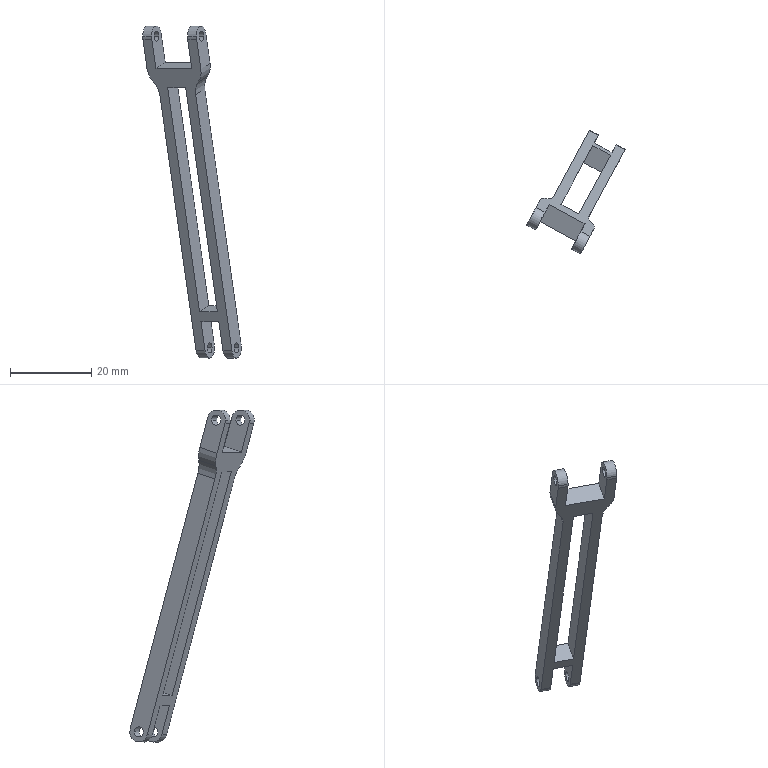Part | SolidWorks | features ICE 7, HoleWzd 4, Extrusion 1 | 1 solid | 34 faces | box 24.253 x 30.565 x 81.628 mm | volume 2325 mm3 | cylinder 18 | plane 16 | commonest cylinder face diameters 2.5 x8 5 x6 10 x4
STEP:
#1=CARTESIAN_POINT('',(-37.304,-81.964,-265.344));
#2=VERTEX_POINT('',#1);
#3=CARTESIAN_POINT('',(-38.488,-84.166,-265.344));
#4=VERTEX_POINT('',#3);
#5=CARTESIAN_POINT('',(-37.896,-83.065,-265.344));
#6=DIRECTION('',(-0.8809,0.4732,0.));
#7=DIRECTION('',(-0.4732,-0.8809,0.));
#8=AXIS2_PLACEMENT_3D('',#5,#6,#7);
#9=CIRCLE('',#8,1.25);
#10=EDGE_CURVE('',#2,#4,#9,.T.);
#11=ORIENTED_EDGE('',*,*,#10,.T.);
#12=CARTESIAN_POINT('',(-36.285,-85.349,-265.344));
#13=VERTEX_POINT('',#12);
#14=CARTESIAN_POINT('',(-36.285,-85.349,-265.344));
#15=DIRECTION('',(0.8809,-0.4732,0.));
#16=VECTOR('',#15,1000.);
#17=LINE('',#14,#16);
#18=EDGE_CURVE('',#4,#13,#17,.T.);
#19=ORIENTED_EDGE('',*,*,#18,.T.);
#20=CARTESIAN_POINT('',(-35.102,-83.147,-265.344));
#21=VERTEX_POINT('',#20);
#22=CARTESIAN_POINT('',(-35.694,-84.248,-265.344));
#23=DIRECTION('',(-0.8809,0.4732,0.));
#24=DIRECTION('',(-0.4732,-0.8809,0.));
#25=AXIS2_PLACEMENT_3D('',#22,#23,#24);
#26=CIRCLE('',#25,1.25);
#27=EDGE_CURVE('',#21,#13,#26,.T.);
#28=ORIENTED_EDGE('',*,*,#27,.F.);
#29=CARTESIAN_POINT('',(-35.102,-83.147,-265.344));
#30=DIRECTION('',(0.8809,-0.4732,0.));
#31=VECTOR('',#30,1000.);
#32=LINE('',#29,#31);
#33=EDGE_CURVE('',#2,#21,#32,.T.);
#34=ORIENTED_EDGE('',*,*,#33,.F.);
#35=EDGE_LOOP('',(#11,#19,#28,#34));
#36=FACE_OUTER_BOUND('',#35,.T.);
#37=CARTESIAN_POINT('',(-35.694,-84.248,-265.344));
#38=DIRECTION('',(0.8809,-0.4732,0.));
#39=DIRECTION('',(0.4732,0.8809,0.));
#40=AXIS2_PLACEMENT_3D('',#37,#38,#39);
#41=CYLINDRICAL_SURFACE('',#40,1.25);
#42=ADVANCED_FACE('',(#36),#41,.F.);
#43=CARTESIAN_POINT('',(-27.476,-90.082,-265.344));
#44=VERTEX_POINT('',#43);
#45=CARTESIAN_POINT('',(-26.293,-87.879,-265.344));
#46=VERTEX_POINT('',#45);
#47=CARTESIAN_POINT('',(-26.884,-88.981,-265.344));
#48=DIRECTION('',(0.8809,-0.4732,0.));
#49=DIRECTION('',(0.4732,0.8809,0.));
#50=AXIS2_PLACEMENT_3D('',#47,#48,#49);
#51=CIRCLE('',#50,1.25);
#52=EDGE_CURVE('',#44,#46,#51,.T.);
#53=ORIENTED_EDGE('',*,*,#52,.F.);
#54=CARTESIAN_POINT('',(-25.274,-91.265,-265.344));
#55=VERTEX_POINT('',#54);
#56=CARTESIAN_POINT('',(-25.274,-91.265,-265.344));
#57=DIRECTION('',(0.8809,-0.4732,0.));
#58=VECTOR('',#57,1000.);
#59=LINE('',#56,#58);
#60=EDGE_CURVE('',#44,#55,#59,.T.);
#61=ORIENTED_EDGE('',*,*,#60,.T.);
#62=CARTESIAN_POINT('',(-24.09,-89.063,-265.344));
#63=VERTEX_POINT('',#62);
#64=CARTESIAN_POINT('',(-24.682,-90.164,-265.344));
#65=DIRECTION('',(0.8809,-0.4732,0.));
#66=DIRECTION('',(0.4732,0.8809,0.));
#67=AXIS2_PLACEMENT_3D('',#64,#65,#66);
#68=CIRCLE('',#67,1.25);
#69=EDGE_CURVE('',#55,#63,#68,.T.);
#70=ORIENTED_EDGE('',*,*,#69,.T.);
#71=CARTESIAN_POINT('',(-24.09,-89.063,-265.344));
#72=DIRECTION('',(0.8809,-0.4732,0.));
#73=VECTOR('',#72,1000.);
#74=LINE('',#71,#73);
#75=EDGE_CURVE('',#46,#63,#74,.T.);
#76=ORIENTED_EDGE('',*,*,#75,.F.);
#77=EDGE_LOOP('',(#53,#61,#70,#76));
#78=FACE_OUTER_BOUND('',#77,.T.);
#79=CARTESIAN_POINT('',(-24.682,-90.164,-265.344));
#80=DIRECTION('',(0.8809,-0.4732,0.));
#81=DIRECTION('',(0.4732,0.8809,0.));
#82=AXIS2_PLACEMENT_3D('',#79,#80,#81);
#83=CYLINDRICAL_SURFACE('',#82,1.25);
#84=ADVANCED_FACE('',(#78),#83,.F.);
#85=CARTESIAN_POINT('',(-25.41,-65.105,-341.972));
#86=VERTEX_POINT('',#85);
#87=CARTESIAN_POINT('',(-24.227,-62.902,-341.972));
#88=VERTEX_POINT('',#87);
#89=CARTESIAN_POINT('',(-24.818,-64.003,-341.972));
#90=DIRECTION('',(0.8809,-0.4732,0.));
#91=DIRECTION('',(0.4732,0.8809,0.));
#92=AXIS2_PLACEMENT_3D('',#89,#90,#91);
#93=CIRCLE('',#92,1.25);
#94=EDGE_CURVE('',#86,#88,#93,.T.);
#95=ORIENTED_EDGE('',*,*,#94,.F.);
#96=CARTESIAN_POINT('',(-23.207,-66.288,-341.972));
#97=VERTEX_POINT('',#96);
#98=CARTESIAN_POINT('',(-23.207,-66.288,-341.972));
#99=DIRECTION('',(0.8809,-0.4732,0.));
#100=VECTOR('',#99,1000.);
#101=LINE('',#98,#100);
#102=EDGE_CURVE('',#86,#97,#101,.T.);
#103=ORIENTED_EDGE('',*,*,#102,.T.);
#104=CARTESIAN_POINT('',(-22.024,-64.085,-341.972));
#105=VERTEX_POINT('',#104);
#106=CARTESIAN_POINT('',(-22.616,-65.186,-341.972));
#107=DIRECTION('',(0.8809,-0.4732,0.));
#108=DIRECTION('',(0.4732,0.8809,0.));
#109=AXIS2_PLACEMENT_3D('',#106,#107,#108);
#110=CIRCLE('',#109,1.25);
#111=EDGE_CURVE('',#97,#105,#110,.T.);
#112=ORIENTED_EDGE('',*,*,#111,.T.);
#113=CARTESIAN_POINT('',(-22.024,-64.085,-341.972));
#114=DIRECTION('',(0.8809,-0.4732,0.));
#115=VECTOR('',#114,1000.);
#116=LINE('',#113,#115);
#117=EDGE_CURVE('',#88,#105,#116,.T.);
#118=ORIENTED_EDGE('',*,*,#117,.F.);
#119=EDGE_LOOP('',(#95,#103,#112,#118));
#120=FACE_OUTER_BOUND('',#119,.T.);
#121=CARTESIAN_POINT('',(-22.616,-65.186,-341.972));
#122=DIRECTION('',(0.8809,-0.4732,0.));
#123=DIRECTION('',(0.4732,0.8809,0.));
#124=AXIS2_PLACEMENT_3D('',#121,#122,#123);
#125=CYLINDRICAL_SURFACE('',#124,1.25);
#126=ADVANCED_FACE('',(#120),#125,.F.);
#127=CARTESIAN_POINT('',(-18.803,-68.654,-341.972));
#128=VERTEX_POINT('',#127);
#129=CARTESIAN_POINT('',(-17.62,-66.452,-341.972));
#130=VERTEX_POINT('',#129);
#131=CARTESIAN_POINT('',(-18.211,-67.553,-341.972));
#132=DIRECTION('',(0.8809,-0.4732,0.));
#133=DIRECTION('',(0.4732,0.8809,0.));
#134=AXIS2_PLACEMENT_3D('',#131,#132,#133);
#135=CIRCLE('',#134,1.25);
#136=EDGE_CURVE('',#128,#130,#135,.T.);
#137=ORIENTED_EDGE('',*,*,#136,.F.);
#138=CARTESIAN_POINT('',(-16.6,-69.837,-341.972));
#139=VERTEX_POINT('',#138);
#140=CARTESIAN_POINT('',(-16.6,-69.837,-341.972));
#141=DIRECTION('',(0.8809,-0.4732,0.));
#142=VECTOR('',#141,1000.);
#143=LINE('',#140,#142);
#144=EDGE_CURVE('',#128,#139,#143,.T.);
#145=ORIENTED_EDGE('',*,*,#144,.T.);
#146=CARTESIAN_POINT('',(-15.417,-67.635,-341.972));
#147=VERTEX_POINT('',#146);
#148=CARTESIAN_POINT('',(-16.009,-68.736,-341.972));
#149=DIRECTION('',(0.8809,-0.4732,0.));
#150=DIRECTION('',(0.4732,0.8809,0.));
#151=AXIS2_PLACEMENT_3D('',#148,#149,#150);
#152=CIRCLE('',#151,1.25);
#153=EDGE_CURVE('',#139,#147,#152,.T.);
#154=ORIENTED_EDGE('',*,*,#153,.T.);
#155=CARTESIAN_POINT('',(-15.417,-67.635,-341.972));
#156=DIRECTION('',(0.8809,-0.4732,0.));
#157=VECTOR('',#156,1000.);
#158=LINE('',#155,#157);
#159=EDGE_CURVE('',#130,#147,#158,.T.);
#160=ORIENTED_EDGE('',*,*,#159,.F.);
#161=EDGE_LOOP('',(#137,#145,#154,#160));
#162=FACE_OUTER_BOUND('',#161,.T.);
#163=CARTESIAN_POINT('',(-16.009,-68.736,-341.972));
#164=DIRECTION('',(0.8809,-0.4732,0.));
#165=DIRECTION('',(0.4732,0.8809,0.));
#166=AXIS2_PLACEMENT_3D('',#163,#164,#165);
#167=CYLINDRICAL_SURFACE('',#166,1.25);
#168=ADVANCED_FACE('',(#162),#167,.F.);
#169=CARTESIAN_POINT('',(-25.815,-92.273,-266.062));
#170=VERTEX_POINT('',#169);
#171=CARTESIAN_POINT('',(-25.865,-92.366,-265.344));
#172=VERTEX_POINT('',#171);
#173=CARTESIAN_POINT('',(-24.682,-90.164,-265.344));
#174=DIRECTION('',(-0.8809,0.4732,0.));
#175=DIRECTION('',(-0.4732,-0.8809,0.));
#176=AXIS2_PLACEMENT_3D('',#173,#174,#175);
#177=CIRCLE('',#176,2.5);
#178=EDGE_CURVE('',#170,#172,#177,.T.);
#179=ORIENTED_EDGE('',*,*,#178,.T.);
#180=CARTESIAN_POINT('',(-28.067,-91.183,-265.344));
#181=VERTEX_POINT('',#180);
#182=CARTESIAN_POINT('',(-25.865,-92.366,-265.344));
#183=DIRECTION('',(-0.8809,0.4732,0.));
#184=VECTOR('',#183,1000.);
#185=LINE('',#182,#184);
#186=EDGE_CURVE('',#172,#181,#185,.T.);
#187=ORIENTED_EDGE('',*,*,#186,.T.);
#188=CARTESIAN_POINT('',(-28.018,-91.09,-266.062));
#189=VERTEX_POINT('',#188);
#190=CARTESIAN_POINT('',(-26.884,-88.981,-265.344));
#191=DIRECTION('',(-0.8809,0.4732,0.));
#192=DIRECTION('',(0.4732,0.8809,0.));
#193=AXIS2_PLACEMENT_3D('',#190,#191,#192);
#194=CIRCLE('',#193,2.5);
#195=EDGE_CURVE('',#189,#181,#194,.T.);
#196=ORIENTED_EDGE('',*,*,#195,.F.);
#197=CARTESIAN_POINT('',(-25.815,-92.273,-266.062));
#198=DIRECTION('',(-0.8809,0.4732,0.));
#199=VECTOR('',#198,1000.);
#200=LINE('',#197,#199);
#201=EDGE_CURVE('',#170,#189,#200,.T.);
#202=ORIENTED_EDGE('',*,*,#201,.F.);
#203=EDGE_LOOP('',(#179,#187,#196,#202));
#204=FACE_OUTER_BOUND('',#203,.T.);
#205=CARTESIAN_POINT('',(-24.682,-90.164,-265.344));
#206=DIRECTION('',(-0.8809,0.4732,0.));
#207=DIRECTION('',(-0.4732,-0.8809,0.));
#208=AXIS2_PLACEMENT_3D('',#205,#206,#207);
#209=CYLINDRICAL_SURFACE('',#208,2.5);
#210=ADVANCED_FACE('',(#204),#209,.T.);
#211=CARTESIAN_POINT('',(-36.877,-86.451,-265.344));
#212=VERTEX_POINT('',#211);
#213=CARTESIAN_POINT('',(-36.827,-86.358,-266.062));
#214=VERTEX_POINT('',#213);
#215=CARTESIAN_POINT('',(-35.694,-84.248,-265.344));
#216=DIRECTION('',(0.8809,-0.4732,0.));
#217=DIRECTION('',(-0.4732,-0.8809,0.));
#218=AXIS2_PLACEMENT_3D('',#215,#216,#217);
#219=CIRCLE('',#218,2.5);
#220=EDGE_CURVE('',#212,#214,#219,.T.);
#221=ORIENTED_EDGE('',*,*,#220,.F.);
#222=CARTESIAN_POINT('',(-39.079,-85.267,-265.344));
#223=VERTEX_POINT('',#222);
#224=CARTESIAN_POINT('',(-25.865,-92.366,-265.344));
#225=DIRECTION('',(-0.8809,0.4732,0.));
#226=VECTOR('',#225,1000.);
#227=LINE('',#224,#226);
#228=EDGE_CURVE('',#212,#223,#227,.T.);
#229=ORIENTED_EDGE('',*,*,#228,.T.);
#230=CARTESIAN_POINT('',(-39.029,-85.175,-266.062));
#231=VERTEX_POINT('',#230);
#232=CARTESIAN_POINT('',(-37.896,-83.065,-265.344));
#233=DIRECTION('',(-0.8809,0.4732,0.));
#234=DIRECTION('',(-0.4732,-0.8809,0.));
#235=AXIS2_PLACEMENT_3D('',#232,#233,#234);
#236=CIRCLE('',#235,2.5);
#237=EDGE_CURVE('',#231,#223,#236,.T.);
#238=ORIENTED_EDGE('',*,*,#237,.F.);
#239=CARTESIAN_POINT('',(-25.815,-92.273,-266.062));
#240=DIRECTION('',(-0.8809,0.4732,0.));
#241=VECTOR('',#240,1000.);
#242=LINE('',#239,#241);
#243=EDGE_CURVE('',#214,#231,#242,.T.);
#244=ORIENTED_EDGE('',*,*,#243,.F.);
#245=EDGE_LOOP('',(#221,#229,#238,#244));
#246=FACE_OUTER_BOUND('',#245,.T.);
#247=CARTESIAN_POINT('',(-24.682,-90.164,-265.344));
#248=DIRECTION('',(-0.8809,0.4732,0.));
#249=DIRECTION('',(-0.4732,-0.8809,0.));
#250=AXIS2_PLACEMENT_3D('',#247,#248,#249);
#251=CYLINDRICAL_SURFACE('',#250,2.5);
#252=ADVANCED_FACE('',(#246),#251,.T.);
#253=CARTESIAN_POINT('',(-23.749,-67.296,-342.69));
#254=VERTEX_POINT('',#253);
#255=CARTESIAN_POINT('',(-21.483,-63.077,-341.254));
#256=VERTEX_POINT('',#255);
#257=CARTESIAN_POINT('',(-22.616,-65.186,-341.972));
#258=DIRECTION('',(0.8809,-0.4732,0.));
#259=DIRECTION('',(-0.4732,-0.8809,0.));
#260=AXIS2_PLACEMENT_3D('',#257,#258,#259);
#261=CIRCLE('',#260,2.5);
#262=EDGE_CURVE('',#254,#256,#261,.T.);
#263=ORIENTED_EDGE('',*,*,#262,.F.);
#264=CARTESIAN_POINT('',(-25.951,-66.113,-342.69));
#265=VERTEX_POINT('',#264);
#266=CARTESIAN_POINT('',(-14.94,-72.028,-342.69));
#267=DIRECTION('',(-0.8809,0.4732,0.));
#268=VECTOR('',#267,1000.);
#269=LINE('',#266,#268);
#270=EDGE_CURVE('',#254,#265,#269,.T.);
#271=ORIENTED_EDGE('',*,*,#270,.T.);
#272=CARTESIAN_POINT('',(-23.685,-61.894,-341.254));
#273=VERTEX_POINT('',#272);
#274=CARTESIAN_POINT('',(-24.818,-64.003,-341.972));
#275=DIRECTION('',(-0.8809,0.4732,0.));
#276=DIRECTION('',(0.4732,0.8809,0.));
#277=AXIS2_PLACEMENT_3D('',#274,#275,#276);
#278=CIRCLE('',#277,2.5);
#279=EDGE_CURVE('',#273,#265,#278,.T.);
#280=ORIENTED_EDGE('',*,*,#279,.F.);
#281=CARTESIAN_POINT('',(-12.673,-67.809,-341.254));
#282=DIRECTION('',(-0.8809,0.4732,0.));
#283=VECTOR('',#282,1000.);
#284=LINE('',#281,#283);
#285=EDGE_CURVE('',#256,#273,#284,.T.);
#286=ORIENTED_EDGE('',*,*,#285,.F.);
#287=EDGE_LOOP('',(#263,#271,#280,#286));
#288=FACE_OUTER_BOUND('',#287,.T.);
#289=CARTESIAN_POINT('',(-13.806,-69.919,-341.972));
#290=DIRECTION('',(-0.8809,0.4732,0.));
#291=DIRECTION('',(-0.4732,-0.8809,0.));
#292=AXIS2_PLACEMENT_3D('',#289,#290,#291);
#293=CYLINDRICAL_SURFACE('',#292,2.5);
#294=ADVANCED_FACE('',(#288),#293,.T.);
#295=ORIENTED_EDGE('',*,*,#228,.F.);
#296=CARTESIAN_POINT('',(-34.56,-82.139,-264.626));
#297=VERTEX_POINT('',#296);
#298=CARTESIAN_POINT('',(-35.694,-84.248,-265.344));
#299=DIRECTION('',(0.8809,-0.4732,0.));
#300=DIRECTION('',(-0.4732,-0.8809,0.));
#301=AXIS2_PLACEMENT_3D('',#298,#299,#300);
#302=CIRCLE('',#301,2.5);
#303=EDGE_CURVE('',#297,#212,#302,.T.);
#304=ORIENTED_EDGE('',*,*,#303,.F.);
#305=CARTESIAN_POINT('',(-36.763,-80.956,-264.626));
#306=VERTEX_POINT('',#305);
#307=CARTESIAN_POINT('',(-23.549,-88.054,-264.626));
#308=DIRECTION('',(-0.8809,0.4732,0.));
#309=VECTOR('',#308,1000.);
#310=LINE('',#307,#309);
#311=EDGE_CURVE('',#297,#306,#310,.T.);
#312=ORIENTED_EDGE('',*,*,#311,.T.);
#313=CARTESIAN_POINT('',(-37.896,-83.065,-265.344));
#314=DIRECTION('',(-0.8809,0.4732,0.));
#315=DIRECTION('',(-0.4732,-0.8809,0.));
#316=AXIS2_PLACEMENT_3D('',#313,#314,#315);
#317=CIRCLE('',#316,2.5);
#318=EDGE_CURVE('',#223,#306,#317,.T.);
#319=ORIENTED_EDGE('',*,*,#318,.F.);
#320=EDGE_LOOP('',(#295,#304,#312,#319));
#321=FACE_OUTER_BOUND('',#320,.T.);
#322=CARTESIAN_POINT('',(-24.682,-90.164,-265.344));
#323=DIRECTION('',(-0.8809,0.4732,0.));
#324=DIRECTION('',(-0.4732,-0.8809,0.));
#325=AXIS2_PLACEMENT_3D('',#322,#323,#324);
#326=CYLINDRICAL_SURFACE('',#325,2.5);
#327=ADVANCED_FACE('',(#321),#326,.T.);
#328=CARTESIAN_POINT('',(-24.766,-90.321,-273.453));
#329=VERTEX_POINT('',#328);
#330=CARTESIAN_POINT('',(-14.94,-72.028,-342.69));
#331=DIRECTION('',(-0.1359,-0.2531,0.9579));
#332=VECTOR('',#331,1000.);
#333=LINE('',#330,#332);
#334=EDGE_CURVE('',#329,#170,#333,.T.);
#335=ORIENTED_EDGE('',*,*,#334,.F.);
#336=CARTESIAN_POINT('',(-22.5,-86.102,-272.016));
#337=VERTEX_POINT('',#336);
#338=CARTESIAN_POINT('',(-9.529,-61.956,-263.796));
#339=DIRECTION('',(0.4533,0.8438,0.2873));
#340=VECTOR('',#339,1000.);
#341=LINE('',#338,#340);
#342=EDGE_CURVE('',#329,#337,#341,.T.);
#343=ORIENTED_EDGE('',*,*,#342,.T.);
#344=CARTESIAN_POINT('',(-23.549,-88.054,-264.626));
#345=VERTEX_POINT('',#344);
#346=CARTESIAN_POINT('',(-23.549,-88.054,-264.626));
#347=DIRECTION('',(0.1359,0.2531,-0.9579));
#348=VECTOR('',#347,1000.);
#349=LINE('',#346,#348);
#350=EDGE_CURVE('',#345,#337,#349,.T.);
#351=ORIENTED_EDGE('',*,*,#350,.F.);
#352=CARTESIAN_POINT('',(-24.682,-90.164,-265.344));
#353=DIRECTION('',(-0.8809,0.4732,0.));
#354=DIRECTION('',(-0.4732,-0.8809,0.));
#355=AXIS2_PLACEMENT_3D('',#352,#353,#354);
#356=CIRCLE('',#355,2.5);
#357=EDGE_CURVE('',#172,#345,#356,.T.);
#358=ORIENTED_EDGE('',*,*,#357,.F.);
#359=ORIENTED_EDGE('',*,*,#178,.F.);
#360=EDGE_LOOP('',(#335,#343,#351,#358,#359));
#361=FACE_OUTER_BOUND('',#360,.T.);
#362=CARTESIAN_POINT('',(-24.682,-90.164,-265.344));
#363=DIRECTION('',(0.8809,-0.4732,0.));
#364=DIRECTION('',(0.4732,0.8809,0.));
#365=AXIS2_PLACEMENT_3D('',#362,#363,#364);
#366=CIRCLE('',#365,1.25);
#367=EDGE_CURVE('',#63,#55,#366,.T.);
#368=ORIENTED_EDGE('',*,*,#367,.F.);
#369=ORIENTED_EDGE('',*,*,#69,.F.);
#370=EDGE_LOOP('',(#368,#369));
#371=FACE_BOUND('',#370,.T.);
#372=CARTESIAN_POINT('',(-24.682,-90.164,-265.344));
#373=DIRECTION('',(-0.8809,0.4732,0.));
#374=DIRECTION('',(-0.4732,-0.8809,0.));
#375=AXIS2_PLACEMENT_3D('',#372,#373,#374);
#376=PLANE('',#375);
#377=ADVANCED_FACE('',(#361,#371),#376,.F.);
#378=CARTESIAN_POINT('',(-32.925,-84.378,-278.035));
#379=VERTEX_POINT('',#378);
#380=CARTESIAN_POINT('',(-25.109,-69.827,-333.112));
#381=VERTEX_POINT('',#380);
#382=CARTESIAN_POINT('',(-32.925,-84.378,-278.035));
#383=DIRECTION('',(0.1359,0.2531,-0.9579));
#384=VECTOR('',#383,1000.);
#385=LINE('',#382,#384);
#386=EDGE_CURVE('',#379,#381,#385,.T.);
#387=ORIENTED_EDGE('',*,*,#386,.F.);
#388=CARTESIAN_POINT('',(-28.521,-86.744,-278.035));
#389=VERTEX_POINT('',#388);
#390=CARTESIAN_POINT('',(-28.521,-86.744,-278.035));
#391=DIRECTION('',(-0.8809,0.4732,0.));
#392=VECTOR('',#391,1000.);
#393=LINE('',#390,#392);
#394=EDGE_CURVE('',#389,#379,#393,.T.);
#395=ORIENTED_EDGE('',*,*,#394,.F.);
#396=CARTESIAN_POINT('',(-20.704,-72.193,-333.112));
#397=VERTEX_POINT('',#396);
#398=CARTESIAN_POINT('',(-20.704,-72.193,-333.112));
#399=DIRECTION('',(-0.1359,-0.2531,0.9579));
#400=VECTOR('',#399,1000.);
#401=LINE('',#398,#400);
#402=EDGE_CURVE('',#397,#389,#401,.T.);
#403=ORIENTED_EDGE('',*,*,#402,.F.);
#404=CARTESIAN_POINT('',(-25.109,-69.827,-333.112));
#405=DIRECTION('',(0.8809,-0.4732,0.));
#406=VECTOR('',#405,1000.);
#407=LINE('',#404,#406);
#408=EDGE_CURVE('',#381,#397,#407,.T.);
#409=ORIENTED_EDGE('',*,*,#408,.F.);
#410=EDGE_LOOP('',(#387,#395,#403,#409));
#411=FACE_BOUND('',#410,.T.);
#412=CARTESIAN_POINT('',(-26.069,-87.464,-279.788));
#413=VERTEX_POINT('',#412);
#414=CARTESIAN_POINT('',(-17.142,-70.845,-342.69));
#415=VERTEX_POINT('',#414);
#416=CARTESIAN_POINT('',(-26.069,-87.464,-279.788));
#417=DIRECTION('',(0.1359,0.2531,-0.9579));
#418=VECTOR('',#417,1000.);
#419=LINE('',#416,#418);
#420=EDGE_CURVE('',#413,#415,#419,.T.);
#421=ORIENTED_EDGE('',*,*,#420,.F.);
#422=CARTESIAN_POINT('',(-25.418,-88.892,-276.62));
#423=VERTEX_POINT('',#422);
#424=CARTESIAN_POINT('',(-21.665,-89.83,-279.788));
#425=DIRECTION('',(-0.4533,-0.8438,-0.2873));
#426=DIRECTION('',(0.8809,-0.4732,0.));
#427=AXIS2_PLACEMENT_3D('',#424,#425,#426);
#428=CIRCLE('',#427,5.);
#429=EDGE_CURVE('',#423,#413,#428,.T.);
#430=ORIENTED_EDGE('',*,*,#429,.F.);
#431=CARTESIAN_POINT('',(-29.171,-87.954,-273.453));
#432=DIRECTION('',(0.4533,0.8438,0.2873));
#433=DIRECTION('',(-0.8809,0.4732,0.));
#434=AXIS2_PLACEMENT_3D('',#431,#432,#433);
#435=CIRCLE('',#434,5.);
#436=EDGE_CURVE('',#329,#423,#435,.T.);
#437=ORIENTED_EDGE('',*,*,#436,.F.);
#438=ORIENTED_EDGE('',*,*,#334,.T.);
#439=ORIENTED_EDGE('',*,*,#201,.T.);
#440=CARTESIAN_POINT('',(-26.998,-89.192,-273.246));
#441=VERTEX_POINT('',#440);
#442=CARTESIAN_POINT('',(-26.998,-89.192,-273.246));
#443=DIRECTION('',(-0.1359,-0.2531,0.9579));
#444=VECTOR('',#443,1000.);
#445=LINE('',#442,#444);
#446=EDGE_CURVE('',#441,#189,#445,.T.);
#447=ORIENTED_EDGE('',*,*,#446,.F.);
#448=CARTESIAN_POINT('',(-35.807,-84.46,-273.246));
#449=VERTEX_POINT('',#448);
#450=CARTESIAN_POINT('',(-35.807,-84.46,-273.246));
#451=DIRECTION('',(0.8809,-0.4732,0.));
#452=VECTOR('',#451,1000.);
#453=LINE('',#450,#452);
#454=EDGE_CURVE('',#449,#441,#453,.T.);
#455=ORIENTED_EDGE('',*,*,#454,.F.);
#456=CARTESIAN_POINT('',(-36.827,-86.358,-266.062));
#457=DIRECTION('',(0.1359,0.2531,-0.9579));
#458=VECTOR('',#457,1000.);
#459=LINE('',#456,#458);
#460=EDGE_CURVE('',#214,#449,#459,.T.);
#461=ORIENTED_EDGE('',*,*,#460,.F.);
#462=ORIENTED_EDGE('',*,*,#243,.T.);
#463=CARTESIAN_POINT('',(-37.98,-83.222,-273.453));
#464=VERTEX_POINT('',#463);
#465=CARTESIAN_POINT('',(-28.154,-64.93,-342.69));
#466=DIRECTION('',(-0.1359,-0.2531,0.9579));
#467=VECTOR('',#466,1000.);
#468=LINE('',#465,#467);
#469=EDGE_CURVE('',#464,#231,#468,.T.);
#470=ORIENTED_EDGE('',*,*,#469,.F.);
#471=CARTESIAN_POINT('',(-36.43,-82.977,-276.62));
#472=VERTEX_POINT('',#471);
#473=CARTESIAN_POINT('',(-33.576,-85.588,-273.453));
#474=DIRECTION('',(0.4533,0.8438,0.2873));
#475=DIRECTION('',(-0.8809,0.4732,0.));
#476=AXIS2_PLACEMENT_3D('',#473,#474,#475);
#477=CIRCLE('',#476,5.);
#478=EDGE_CURVE('',#472,#464,#477,.T.);
#479=ORIENTED_EDGE('',*,*,#478,.F.);
#480=CARTESIAN_POINT('',(-34.879,-82.731,-279.788));
#481=VERTEX_POINT('',#480);
#482=CARTESIAN_POINT('',(-39.283,-80.365,-279.788));
#483=DIRECTION('',(-0.4533,-0.8438,-0.2873));
#484=DIRECTION('',(0.8809,-0.4732,0.));
#485=AXIS2_PLACEMENT_3D('',#482,#483,#484);
#486=CIRCLE('',#485,5.);
#487=EDGE_CURVE('',#481,#472,#486,.T.);
#488=ORIENTED_EDGE('',*,*,#487,.F.);
#489=CARTESIAN_POINT('',(-25.951,-66.113,-342.69));
#490=DIRECTION('',(-0.1359,-0.2531,0.9579));
#491=VECTOR('',#490,1000.);
#492=LINE('',#489,#491);
#493=EDGE_CURVE('',#265,#481,#492,.T.);
#494=ORIENTED_EDGE('',*,*,#493,.F.);
#495=ORIENTED_EDGE('',*,*,#270,.F.);
#496=CARTESIAN_POINT('',(-24.769,-69.194,-335.506));
#497=VERTEX_POINT('',#496);
#498=CARTESIAN_POINT('',(-24.769,-69.194,-335.506));
#499=DIRECTION('',(0.1359,0.2531,-0.9579));
#500=VECTOR('',#499,1000.);
#501=LINE('',#498,#500);
#502=EDGE_CURVE('',#497,#254,#501,.T.);
#503=ORIENTED_EDGE('',*,*,#502,.F.);
#504=CARTESIAN_POINT('',(-20.364,-71.56,-335.506));
#505=VERTEX_POINT('',#504);
#506=CARTESIAN_POINT('',(-20.364,-71.56,-335.506));
#507=DIRECTION('',(-0.8809,0.4732,0.));
#508=VECTOR('',#507,1000.);
#509=LINE('',#506,#508);
#510=EDGE_CURVE('',#505,#497,#509,.T.);
#511=ORIENTED_EDGE('',*,*,#510,.F.);
#512=CARTESIAN_POINT('',(-19.344,-69.662,-342.69));
#513=VERTEX_POINT('',#512);
#514=CARTESIAN_POINT('',(-19.344,-69.662,-342.69));
#515=DIRECTION('',(-0.1359,-0.2531,0.9579));
#516=VECTOR('',#515,1000.);
#517=LINE('',#514,#516);
#518=EDGE_CURVE('',#513,#505,#517,.T.);
#519=ORIENTED_EDGE('',*,*,#518,.F.);
#520=CARTESIAN_POINT('',(-14.94,-72.028,-342.69));
#521=DIRECTION('',(-0.8809,0.4732,0.));
#522=VECTOR('',#521,1000.);
#523=LINE('',#520,#522);
#524=EDGE_CURVE('',#415,#513,#523,.T.);
#525=ORIENTED_EDGE('',*,*,#524,.F.);
#526=EDGE_LOOP('',(#421,#430,#437,#438,#439,#447,#455,#461,#462,#470,#479,#488,#494,#495,#503,#511,#519,#525));
#527=FACE_OUTER_BOUND('',#526,.T.);
#528=CARTESIAN_POINT('',(-14.94,-72.028,-342.69));
#529=DIRECTION('',(-0.4533,-0.8438,-0.2873));
#530=DIRECTION('',(0.8809,-0.4732,0.));
#531=AXIS2_PLACEMENT_3D('',#528,#529,#530);
#532=PLANE('',#531);
#533=ADVANCED_FACE('',(#411,#527),#532,.T.);
#534=CARTESIAN_POINT('',(-22.842,-65.608,-331.675));
#535=VERTEX_POINT('',#534);
#536=CARTESIAN_POINT('',(-30.659,-80.159,-276.599));
#537=VERTEX_POINT('',#536);
#538=CARTESIAN_POINT('',(-32.358,-83.322,-264.626));
#539=DIRECTION('',(-0.1359,-0.2531,0.9579));
#540=VECTOR('',#539,1000.);
#541=LINE('',#538,#540);
#542=EDGE_CURVE('',#535,#537,#541,.T.);
#543=ORIENTED_EDGE('',*,*,#542,.F.);
#544=CARTESIAN_POINT('',(-18.437,-67.974,-331.675));
#545=VERTEX_POINT('',#544);
#546=CARTESIAN_POINT('',(-14.033,-70.34,-331.675));
#547=DIRECTION('',(-0.8809,0.4732,0.));
#548=VECTOR('',#547,1000.);
#549=LINE('',#546,#548);
#550=EDGE_CURVE('',#545,#535,#549,.T.);
#551=ORIENTED_EDGE('',*,*,#550,.F.);
#552=CARTESIAN_POINT('',(-26.254,-82.525,-276.599));
#553=VERTEX_POINT('',#552);
#554=CARTESIAN_POINT('',(-27.953,-85.688,-264.626));
#555=DIRECTION('',(0.1359,0.2531,-0.9579));
#556=VECTOR('',#555,1000.);
#557=LINE('',#554,#556);
#558=EDGE_CURVE('',#553,#545,#557,.T.);
#559=ORIENTED_EDGE('',*,*,#558,.F.);
#560=CARTESIAN_POINT('',(-21.849,-84.891,-276.599));
#561=DIRECTION('',(0.8809,-0.4732,0.));
#562=VECTOR('',#561,1000.);
#563=LINE('',#560,#562);
#564=EDGE_CURVE('',#537,#553,#563,.T.);
#565=ORIENTED_EDGE('',*,*,#564,.F.);
#566=EDGE_LOOP('',(#543,#551,#559,#565));
#567=FACE_BOUND('',#566,.T.);
#568=CARTESIAN_POINT('',(-14.876,-66.626,-341.254));
#569=VERTEX_POINT('',#568);
#570=CARTESIAN_POINT('',(-23.803,-83.245,-278.352));
#571=VERTEX_POINT('',#570);
#572=CARTESIAN_POINT('',(-25.751,-86.871,-264.626));
#573=DIRECTION('',(-0.1359,-0.2531,0.9579));
#574=VECTOR('',#573,1000.);
#575=LINE('',#572,#574);
#576=EDGE_CURVE('',#569,#571,#575,.T.);
#577=ORIENTED_EDGE('',*,*,#576,.F.);
#578=CARTESIAN_POINT('',(-17.078,-65.443,-341.254));
#579=VERTEX_POINT('',#578);
#580=CARTESIAN_POINT('',(-12.673,-67.809,-341.254));
#581=DIRECTION('',(-0.8809,0.4732,0.));
#582=VECTOR('',#581,1000.);
#583=LINE('',#580,#582);
#584=EDGE_CURVE('',#569,#579,#583,.T.);
#585=ORIENTED_EDGE('',*,*,#584,.T.);
#586=CARTESIAN_POINT('',(-18.098,-67.341,-334.07));
#587=VERTEX_POINT('',#586);
#588=CARTESIAN_POINT('',(-27.953,-85.688,-264.626));
#589=DIRECTION('',(0.1359,0.2531,-0.9579));
#590=VECTOR('',#589,1000.);
#591=LINE('',#588,#590);
#592=EDGE_CURVE('',#587,#579,#591,.T.);
#593=ORIENTED_EDGE('',*,*,#592,.F.);
#594=CARTESIAN_POINT('',(-22.502,-64.975,-334.07));
#595=VERTEX_POINT('',#594);
#596=CARTESIAN_POINT('',(-13.693,-69.707,-334.07));
#597=DIRECTION('',(0.8809,-0.4732,0.));
#598=VECTOR('',#597,1000.);
#599=LINE('',#596,#598);
#600=EDGE_CURVE('',#595,#587,#599,.T.);
#601=ORIENTED_EDGE('',*,*,#600,.F.);
#602=CARTESIAN_POINT('',(-32.358,-83.322,-264.626));
#603=DIRECTION('',(-0.1359,-0.2531,0.9579));
#604=VECTOR('',#603,1000.);
#605=LINE('',#602,#604);
#606=EDGE_CURVE('',#256,#595,#605,.T.);
#607=ORIENTED_EDGE('',*,*,#606,.F.);
#608=ORIENTED_EDGE('',*,*,#285,.T.);
#609=CARTESIAN_POINT('',(-32.612,-78.512,-278.352));
#610=VERTEX_POINT('',#609);
#611=CARTESIAN_POINT('',(-34.56,-82.139,-264.626));
#612=DIRECTION('',(0.1359,0.2531,-0.9579));
#613=VECTOR('',#612,1000.);
#614=LINE('',#611,#613);
#615=EDGE_CURVE('',#610,#273,#614,.T.);
#616=ORIENTED_EDGE('',*,*,#615,.F.);
#617=CARTESIAN_POINT('',(-34.163,-78.758,-275.184));
#618=VERTEX_POINT('',#617);
#619=CARTESIAN_POINT('',(-37.017,-76.146,-278.352));
#620=DIRECTION('',(0.4533,0.8438,0.2873));
#621=DIRECTION('',(-0.8809,0.4732,0.));
#622=AXIS2_PLACEMENT_3D('',#619,#620,#621);
#623=CIRCLE('',#622,5.);
#624=EDGE_CURVE('',#618,#610,#623,.T.);
#625=ORIENTED_EDGE('',*,*,#624,.F.);
#626=CARTESIAN_POINT('',(-35.714,-79.003,-272.016));
#627=VERTEX_POINT('',#626);
#628=CARTESIAN_POINT('',(-31.309,-81.369,-272.016));
#629=DIRECTION('',(-0.4533,-0.8438,-0.2873));
#630=DIRECTION('',(-0.8809,0.4732,0.));
#631=AXIS2_PLACEMENT_3D('',#628,#629,#630);
#632=CIRCLE('',#631,5.);
#633=EDGE_CURVE('',#627,#618,#632,.T.);
#634=ORIENTED_EDGE('',*,*,#633,.F.);
#635=CARTESIAN_POINT('',(-36.763,-80.956,-264.626));
#636=DIRECTION('',(0.1359,0.2531,-0.9579));
#637=VECTOR('',#636,1000.);
#638=LINE('',#635,#637);
#639=EDGE_CURVE('',#306,#627,#638,.T.);
#640=ORIENTED_EDGE('',*,*,#639,.F.);
#641=ORIENTED_EDGE('',*,*,#311,.F.);
#642=CARTESIAN_POINT('',(-33.541,-80.241,-271.81));
#643=VERTEX_POINT('',#642);
#644=CARTESIAN_POINT('',(-34.56,-82.139,-264.626));
#645=DIRECTION('',(-0.1359,-0.2531,0.9579));
#646=VECTOR('',#645,1000.);
#647=LINE('',#644,#646);
#648=EDGE_CURVE('',#643,#297,#647,.T.);
#649=ORIENTED_EDGE('',*,*,#648,.F.);
#650=CARTESIAN_POINT('',(-24.732,-84.973,-271.81));
#651=VERTEX_POINT('',#650);
#652=CARTESIAN_POINT('',(-22.529,-86.156,-271.81));
#653=DIRECTION('',(-0.8809,0.4732,0.));
#654=VECTOR('',#653,1000.);
#655=LINE('',#652,#654);
#656=EDGE_CURVE('',#651,#643,#655,.T.);
#657=ORIENTED_EDGE('',*,*,#656,.F.);
#658=CARTESIAN_POINT('',(-25.751,-86.871,-264.626));
#659=VERTEX_POINT('',#658);
#660=CARTESIAN_POINT('',(-25.751,-86.871,-264.626));
#661=DIRECTION('',(0.1359,0.2531,-0.9579));
#662=VECTOR('',#661,1000.);
#663=LINE('',#660,#662);
#664=EDGE_CURVE('',#659,#651,#663,.T.);
#665=ORIENTED_EDGE('',*,*,#664,.F.);
#666=CARTESIAN_POINT('',(-23.549,-88.054,-264.626));
#667=DIRECTION('',(-0.8809,0.4732,0.));
#668=VECTOR('',#667,1000.);
#669=LINE('',#666,#668);
#670=EDGE_CURVE('',#345,#659,#669,.T.);
#671=ORIENTED_EDGE('',*,*,#670,.F.);
#672=ORIENTED_EDGE('',*,*,#350,.T.);
#673=CARTESIAN_POINT('',(-23.151,-84.673,-275.184));
#674=VERTEX_POINT('',#673);
#675=CARTESIAN_POINT('',(-26.905,-83.735,-272.016));
#676=DIRECTION('',(-0.4533,-0.8438,-0.2873));
#677=DIRECTION('',(-0.8809,0.4732,0.));
#678=AXIS2_PLACEMENT_3D('',#675,#676,#677);
#679=CIRCLE('',#678,5.);
#680=EDGE_CURVE('',#674,#337,#679,.T.);
#681=ORIENTED_EDGE('',*,*,#680,.F.);
#682=CARTESIAN_POINT('',(-19.398,-85.611,-278.352));
#683=DIRECTION('',(0.4533,0.8438,0.2873));
#684=DIRECTION('',(-0.8809,0.4732,0.));
#685=AXIS2_PLACEMENT_3D('',#682,#683,#684);
#686=CIRCLE('',#685,5.);
#687=EDGE_CURVE('',#571,#674,#686,.T.);
#688=ORIENTED_EDGE('',*,*,#687,.F.);
#689=EDGE_LOOP('',(#577,#585,#593,#601,#607,#608,#616,#625,#634,#640,#641,#649,#657,#665,#671,#672,#681,#688));
#690=FACE_OUTER_BOUND('',#689,.T.);
#691=CARTESIAN_POINT('',(-23.549,-88.054,-264.626));
#692=DIRECTION('',(0.4533,0.8438,0.2873));
#693=DIRECTION('',(-0.8809,0.4732,0.));
#694=AXIS2_PLACEMENT_3D('',#691,#692,#693);
#695=PLANE('',#694);
#696=ADVANCED_FACE('',(#567,#690),#695,.T.);
#697=ORIENTED_EDGE('',*,*,#186,.F.);
#698=ORIENTED_EDGE('',*,*,#357,.T.);
#699=ORIENTED_EDGE('',*,*,#670,.T.);
#700=CARTESIAN_POINT('',(-26.884,-88.981,-265.344));
#701=DIRECTION('',(-0.8809,0.4732,0.));
#702=DIRECTION('',(0.4732,0.8809,0.));
#703=AXIS2_PLACEMENT_3D('',#700,#701,#702);
#704=CIRCLE('',#703,2.5);
#705=EDGE_CURVE('',#181,#659,#704,.T.);
#706=ORIENTED_EDGE('',*,*,#705,.F.);
#707=EDGE_LOOP('',(#697,#698,#699,#706));
#708=FACE_OUTER_BOUND('',#707,.T.);
#709=CARTESIAN_POINT('',(-24.682,-90.164,-265.344));
#710=DIRECTION('',(-0.8809,0.4732,0.));
#711=DIRECTION('',(-0.4732,-0.8809,0.));
#712=AXIS2_PLACEMENT_3D('',#709,#710,#711);
#713=CYLINDRICAL_SURFACE('',#712,2.5);
#714=ADVANCED_FACE('',(#708),#713,.T.);
#715=CARTESIAN_POINT('',(-16.009,-68.736,-341.972));
#716=DIRECTION('',(0.8809,-0.4732,0.));
#717=DIRECTION('',(-0.4732,-0.8809,0.));
#718=AXIS2_PLACEMENT_3D('',#715,#716,#717);
#719=CIRCLE('',#718,2.5);
#720=EDGE_CURVE('',#415,#569,#719,.T.);
#721=ORIENTED_EDGE('',*,*,#720,.F.);
#722=ORIENTED_EDGE('',*,*,#524,.T.);
#723=CARTESIAN_POINT('',(-18.211,-67.553,-341.972));
#724=DIRECTION('',(-0.8809,0.4732,0.));
#725=DIRECTION('',(0.4732,0.8809,0.));
#726=AXIS2_PLACEMENT_3D('',#723,#724,#725);
#727=CIRCLE('',#726,2.5);
#728=EDGE_CURVE('',#579,#513,#727,.T.);
#729=ORIENTED_EDGE('',*,*,#728,.F.);
#730=ORIENTED_EDGE('',*,*,#584,.F.);
#731=EDGE_LOOP('',(#721,#722,#729,#730));
#732=FACE_OUTER_BOUND('',#731,.T.);
#733=CARTESIAN_POINT('',(-13.806,-69.919,-341.972));
#734=DIRECTION('',(-0.8809,0.4732,0.));
#735=DIRECTION('',(-0.4732,-0.8809,0.));
#736=AXIS2_PLACEMENT_3D('',#733,#734,#735);
#737=CYLINDRICAL_SURFACE('',#736,2.5);
#738=ADVANCED_FACE('',(#732),#737,.T.);
#739=ORIENTED_EDGE('',*,*,#10,.F.);
#740=CARTESIAN_POINT('',(-37.896,-83.065,-265.344));
#741=DIRECTION('',(-0.8809,0.4732,0.));
#742=DIRECTION('',(-0.4732,-0.8809,0.));
#743=AXIS2_PLACEMENT_3D('',#740,#741,#742);
#744=CIRCLE('',#743,1.25);
#745=EDGE_CURVE('',#4,#2,#744,.T.);
#746=ORIENTED_EDGE('',*,*,#745,.F.);
#747=EDGE_LOOP('',(#739,#746));
#748=FACE_BOUND('',#747,.T.);
#749=CARTESIAN_POINT('',(-22.743,-54.858,-263.796));
#750=DIRECTION('',(0.4533,0.8438,0.2873));
#751=VECTOR('',#750,1000.);
#752=LINE('',#749,#751);
#753=EDGE_CURVE('',#464,#627,#752,.T.);
#754=ORIENTED_EDGE('',*,*,#753,.F.);
#755=ORIENTED_EDGE('',*,*,#469,.T.);
#756=ORIENTED_EDGE('',*,*,#237,.T.);
#757=ORIENTED_EDGE('',*,*,#318,.T.);
#758=ORIENTED_EDGE('',*,*,#639,.T.);
#759=EDGE_LOOP('',(#754,#755,#756,#757,#758));
#760=FACE_OUTER_BOUND('',#759,.T.);
#761=CARTESIAN_POINT('',(-37.896,-83.065,-265.344));
#762=DIRECTION('',(-0.8809,0.4732,0.));
#763=DIRECTION('',(-0.4732,-0.8809,0.));
#764=AXIS2_PLACEMENT_3D('',#761,#762,#763);
#765=PLANE('',#764);
#766=ADVANCED_FACE('',(#748,#760),#765,.T.);
#767=ORIENTED_EDGE('',*,*,#502,.T.);
#768=ORIENTED_EDGE('',*,*,#262,.T.);
#769=ORIENTED_EDGE('',*,*,#606,.T.);
#770=CARTESIAN_POINT('',(-9.531,-40.829,-325.85));
#771=DIRECTION('',(-0.4533,-0.8438,-0.2873));
#772=VECTOR('',#771,1000.);
#773=LINE('',#770,#772);
#774=EDGE_CURVE('',#595,#497,#773,.T.);
#775=ORIENTED_EDGE('',*,*,#774,.T.);
#776=EDGE_LOOP('',(#767,#768,#769,#775));
#777=FACE_OUTER_BOUND('',#776,.T.);
#778=CARTESIAN_POINT('',(-22.616,-65.186,-341.972));
#779=DIRECTION('',(0.8809,-0.4732,0.));
#780=DIRECTION('',(0.4732,0.8809,0.));
#781=AXIS2_PLACEMENT_3D('',#778,#779,#780);
#782=CIRCLE('',#781,1.25);
#783=EDGE_CURVE('',#105,#97,#782,.T.);
#784=ORIENTED_EDGE('',*,*,#783,.F.);
#785=ORIENTED_EDGE('',*,*,#111,.F.);
#786=EDGE_LOOP('',(#784,#785));
#787=FACE_BOUND('',#786,.T.);
#788=CARTESIAN_POINT('',(-9.531,-40.829,-325.85));
#789=DIRECTION('',(-0.8809,0.4732,0.));
#790=DIRECTION('',(-0.4732,-0.8809,0.));
#791=AXIS2_PLACEMENT_3D('',#788,#789,#790);
#792=PLANE('',#791);
#793=ADVANCED_FACE('',(#777,#787),#792,.F.);
#794=ORIENTED_EDGE('',*,*,#600,.T.);
#795=CARTESIAN_POINT('',(-5.127,-43.196,-325.85));
#796=DIRECTION('',(-0.4533,-0.8438,-0.2873));
#797=VECTOR('',#796,1000.);
#798=LINE('',#795,#797);
#799=EDGE_CURVE('',#587,#505,#798,.T.);
#800=ORIENTED_EDGE('',*,*,#799,.T.);
#801=ORIENTED_EDGE('',*,*,#510,.T.);
#802=ORIENTED_EDGE('',*,*,#774,.F.);
#803=EDGE_LOOP('',(#794,#800,#801,#802));
#804=FACE_OUTER_BOUND('',#803,.T.);
#805=CARTESIAN_POINT('',(-5.127,-43.196,-325.85));
#806=DIRECTION('',(-0.1359,-0.2531,0.9579));
#807=DIRECTION('',(0.,-0.9668,-0.2554));
#808=AXIS2_PLACEMENT_3D('',#805,#806,#807);
#809=PLANE('',#808);
#810=ADVANCED_FACE('',(#804),#809,.F.);
#811=CARTESIAN_POINT('',(-18.211,-67.553,-341.972));
#812=DIRECTION('',(0.8809,-0.4732,0.));
#813=DIRECTION('',(0.4732,0.8809,0.));
#814=AXIS2_PLACEMENT_3D('',#811,#812,#813);
#815=CIRCLE('',#814,1.25);
#816=EDGE_CURVE('',#130,#128,#815,.T.);
#817=ORIENTED_EDGE('',*,*,#816,.T.);
#818=ORIENTED_EDGE('',*,*,#136,.T.);
#819=EDGE_LOOP('',(#817,#818));
#820=FACE_BOUND('',#819,.T.);
#821=ORIENTED_EDGE('',*,*,#592,.T.);
#822=ORIENTED_EDGE('',*,*,#728,.T.);
#823=ORIENTED_EDGE('',*,*,#518,.T.);
#824=ORIENTED_EDGE('',*,*,#799,.F.);
#825=EDGE_LOOP('',(#821,#822,#823,#824));
#826=FACE_OUTER_BOUND('',#825,.T.);
#827=CARTESIAN_POINT('',(-4.107,-41.298,-333.034));
#828=DIRECTION('',(0.8809,-0.4732,0.));
#829=DIRECTION('',(0.4732,0.8809,0.));
#830=AXIS2_PLACEMENT_3D('',#827,#828,#829);
#831=PLANE('',#830);
#832=ADVANCED_FACE('',(#820,#826),#831,.F.);
#833=ORIENTED_EDGE('',*,*,#624,.T.);
#834=CARTESIAN_POINT('',(-19.641,-54.367,-270.132));
#835=DIRECTION('',(-0.4533,-0.8438,-0.2873));
#836=VECTOR('',#835,1000.);
#837=LINE('',#834,#836);
#838=EDGE_CURVE('',#610,#481,#837,.T.);
#839=ORIENTED_EDGE('',*,*,#838,.T.);
#840=ORIENTED_EDGE('',*,*,#487,.T.);
#841=CARTESIAN_POINT('',(-21.192,-54.612,-266.964));
#842=DIRECTION('',(-0.4533,-0.8438,-0.2873));
#843=VECTOR('',#842,1000.);
#844=LINE('',#841,#843);
#845=EDGE_CURVE('',#618,#472,#844,.T.);
#846=ORIENTED_EDGE('',*,*,#845,.F.);
#847=EDGE_LOOP('',(#833,#839,#840,#846));
#848=FACE_OUTER_BOUND('',#847,.T.);
#849=CARTESIAN_POINT('',(-24.046,-52.001,-270.132));
#850=DIRECTION('',(-0.4533,-0.8438,-0.2873));
#851=DIRECTION('',(0.8809,-0.4732,0.));
#852=AXIS2_PLACEMENT_3D('',#849,#850,#851);
#853=CYLINDRICAL_SURFACE('',#852,5.);
#854=ADVANCED_FACE('',(#848),#853,.F.);
#855=CARTESIAN_POINT('',(-24.818,-64.003,-341.972));
#856=DIRECTION('',(0.8809,-0.4732,0.));
#857=DIRECTION('',(0.4732,0.8809,0.));
#858=AXIS2_PLACEMENT_3D('',#855,#856,#857);
#859=CIRCLE('',#858,1.25);
#860=EDGE_CURVE('',#88,#86,#859,.T.);
#861=ORIENTED_EDGE('',*,*,#860,.T.);
#862=ORIENTED_EDGE('',*,*,#94,.T.);
#863=EDGE_LOOP('',(#861,#862));
#864=FACE_BOUND('',#863,.T.);
#865=ORIENTED_EDGE('',*,*,#615,.T.);
#866=ORIENTED_EDGE('',*,*,#279,.T.);
#867=ORIENTED_EDGE('',*,*,#493,.T.);
#868=ORIENTED_EDGE('',*,*,#838,.F.);
#869=EDGE_LOOP('',(#865,#866,#867,#868));
#870=FACE_OUTER_BOUND('',#869,.T.);
#871=CARTESIAN_POINT('',(-10.714,-37.748,-333.034));
#872=DIRECTION('',(0.8809,-0.4732,0.));
#873=DIRECTION('',(0.4732,0.8809,0.));
#874=AXIS2_PLACEMENT_3D('',#871,#872,#873);
#875=PLANE('',#874);
#876=ADVANCED_FACE('',(#864,#870),#875,.F.);
#877=ORIENTED_EDGE('',*,*,#633,.T.);
#878=ORIENTED_EDGE('',*,*,#845,.T.);
#879=ORIENTED_EDGE('',*,*,#478,.T.);
#880=ORIENTED_EDGE('',*,*,#753,.T.);
#881=EDGE_LOOP('',(#877,#878,#879,#880));
#882=FACE_OUTER_BOUND('',#881,.T.);
#883=CARTESIAN_POINT('',(-18.338,-57.224,-263.796));
#884=DIRECTION('',(-0.4533,-0.8438,-0.2873));
#885=DIRECTION('',(0.8809,-0.4732,0.));
#886=AXIS2_PLACEMENT_3D('',#883,#884,#885);
#887=CYLINDRICAL_SURFACE('',#886,5.);
#888=ADVANCED_FACE('',(#882),#887,.T.);
#889=ORIENTED_EDGE('',*,*,#446,.T.);
#890=ORIENTED_EDGE('',*,*,#195,.T.);
#891=ORIENTED_EDGE('',*,*,#705,.T.);
#892=ORIENTED_EDGE('',*,*,#664,.T.);
#893=CARTESIAN_POINT('',(-11.761,-60.828,-263.59));
#894=DIRECTION('',(-0.4533,-0.8438,-0.2873));
#895=VECTOR('',#894,1000.);
#896=LINE('',#893,#895);
#897=EDGE_CURVE('',#651,#441,#896,.T.);
#898=ORIENTED_EDGE('',*,*,#897,.T.);
#899=EDGE_LOOP('',(#889,#890,#891,#892,#898));
#900=FACE_OUTER_BOUND('',#899,.T.);
#901=CARTESIAN_POINT('',(-26.884,-88.981,-265.344));
#902=DIRECTION('',(0.8809,-0.4732,0.));
#903=DIRECTION('',(0.4732,0.8809,0.));
#904=AXIS2_PLACEMENT_3D('',#901,#902,#903);
#905=CIRCLE('',#904,1.25);
#906=EDGE_CURVE('',#46,#44,#905,.T.);
#907=ORIENTED_EDGE('',*,*,#906,.T.);
#908=ORIENTED_EDGE('',*,*,#52,.T.);
#909=EDGE_LOOP('',(#907,#908));
#910=FACE_BOUND('',#909,.T.);
#911=CARTESIAN_POINT('',(-11.761,-60.828,-263.59));
#912=DIRECTION('',(0.8809,-0.4732,0.));
#913=DIRECTION('',(0.4732,0.8809,0.));
#914=AXIS2_PLACEMENT_3D('',#911,#912,#913);
#915=PLANE('',#914);
#916=ADVANCED_FACE('',(#900,#910),#915,.F.);
#917=ORIENTED_EDGE('',*,*,#656,.T.);
#918=CARTESIAN_POINT('',(-20.57,-56.095,-263.59));
#919=DIRECTION('',(-0.4533,-0.8438,-0.2873));
#920=VECTOR('',#919,1000.);
#921=LINE('',#918,#920);
#922=EDGE_CURVE('',#643,#449,#921,.T.);
#923=ORIENTED_EDGE('',*,*,#922,.T.);
#924=ORIENTED_EDGE('',*,*,#454,.T.);
#925=ORIENTED_EDGE('',*,*,#897,.F.);
#926=EDGE_LOOP('',(#917,#923,#924,#925));
#927=FACE_OUTER_BOUND('',#926,.T.);
#928=CARTESIAN_POINT('',(-20.57,-56.095,-263.59));
#929=DIRECTION('',(0.1359,0.2531,-0.9579));
#930=DIRECTION('',(0.,0.9668,0.2554));
#931=AXIS2_PLACEMENT_3D('',#928,#929,#930);
#932=PLANE('',#931);
#933=ADVANCED_FACE('',(#927),#932,.F.);
#934=ORIENTED_EDGE('',*,*,#27,.T.);
#935=CARTESIAN_POINT('',(-35.694,-84.248,-265.344));
#936=DIRECTION('',(-0.8809,0.4732,0.));
#937=DIRECTION('',(-0.4732,-0.8809,0.));
#938=AXIS2_PLACEMENT_3D('',#935,#936,#937);
#939=CIRCLE('',#938,1.25);
#940=EDGE_CURVE('',#13,#21,#939,.T.);
#941=ORIENTED_EDGE('',*,*,#940,.T.);
#942=EDGE_LOOP('',(#934,#941));
#943=FACE_BOUND('',#942,.T.);
#944=ORIENTED_EDGE('',*,*,#648,.T.);
#945=ORIENTED_EDGE('',*,*,#303,.T.);
#946=ORIENTED_EDGE('',*,*,#220,.T.);
#947=ORIENTED_EDGE('',*,*,#460,.T.);
#948=ORIENTED_EDGE('',*,*,#922,.F.);
#949=EDGE_LOOP('',(#944,#945,#946,#947,#948));
#950=FACE_OUTER_BOUND('',#949,.T.);
#951=CARTESIAN_POINT('',(-21.59,-57.993,-256.406));
#952=DIRECTION('',(-0.8809,0.4732,0.));
#953=DIRECTION('',(-0.4732,-0.8809,0.));
#954=AXIS2_PLACEMENT_3D('',#951,#952,#953);
#955=PLANE('',#954);
#956=ADVANCED_FACE('',(#943,#950),#955,.F.);
#957=ORIENTED_EDGE('',*,*,#420,.T.);
#958=ORIENTED_EDGE('',*,*,#720,.T.);
#959=ORIENTED_EDGE('',*,*,#576,.T.);
#960=CARTESIAN_POINT('',(-10.832,-59.099,-270.132));
#961=DIRECTION('',(-0.4533,-0.8438,-0.2873));
#962=VECTOR('',#961,1000.);
#963=LINE('',#960,#962);
#964=EDGE_CURVE('',#571,#413,#963,.T.);
#965=ORIENTED_EDGE('',*,*,#964,.T.);
#966=EDGE_LOOP('',(#957,#958,#959,#965));
#967=FACE_OUTER_BOUND('',#966,.T.);
#968=CARTESIAN_POINT('',(-16.009,-68.736,-341.972));
#969=DIRECTION('',(0.8809,-0.4732,0.));
#970=DIRECTION('',(0.4732,0.8809,0.));
#971=AXIS2_PLACEMENT_3D('',#968,#969,#970);
#972=CIRCLE('',#971,1.25);
#973=EDGE_CURVE('',#147,#139,#972,.T.);
#974=ORIENTED_EDGE('',*,*,#973,.F.);
#975=ORIENTED_EDGE('',*,*,#153,.F.);
#976=EDGE_LOOP('',(#974,#975));
#977=FACE_BOUND('',#976,.T.);
#978=CARTESIAN_POINT('',(-10.832,-59.099,-270.132));
#979=DIRECTION('',(-0.8809,0.4732,0.));
#980=DIRECTION('',(-0.4732,-0.8809,0.));
#981=AXIS2_PLACEMENT_3D('',#978,#979,#980);
#982=PLANE('',#981);
#983=ADVANCED_FACE('',(#967,#977),#982,.F.);
#984=ORIENTED_EDGE('',*,*,#687,.T.);
#985=CARTESIAN_POINT('',(-10.181,-60.528,-266.964));
#986=DIRECTION('',(-0.4533,-0.8438,-0.2873));
#987=VECTOR('',#986,1000.);
#988=LINE('',#985,#987);
#989=EDGE_CURVE('',#674,#423,#988,.T.);
#990=ORIENTED_EDGE('',*,*,#989,.T.);
#991=ORIENTED_EDGE('',*,*,#429,.T.);
#992=ORIENTED_EDGE('',*,*,#964,.F.);
#993=EDGE_LOOP('',(#984,#990,#991,#992));
#994=FACE_OUTER_BOUND('',#993,.T.);
#995=CARTESIAN_POINT('',(-6.427,-61.465,-270.132));
#996=DIRECTION('',(-0.4533,-0.8438,-0.2873));
#997=DIRECTION('',(0.8809,-0.4732,0.));
#998=AXIS2_PLACEMENT_3D('',#995,#996,#997);
#999=CYLINDRICAL_SURFACE('',#998,5.);
#1000=ADVANCED_FACE('',(#994),#999,.F.);
#1001=ORIENTED_EDGE('',*,*,#680,.T.);
#1002=ORIENTED_EDGE('',*,*,#342,.F.);
#1003=ORIENTED_EDGE('',*,*,#436,.T.);
#1004=ORIENTED_EDGE('',*,*,#989,.F.);
#1005=EDGE_LOOP('',(#1001,#1002,#1003,#1004));
#1006=FACE_OUTER_BOUND('',#1005,.T.);
#1007=CARTESIAN_POINT('',(-13.934,-59.59,-263.796));
#1008=DIRECTION('',(-0.4533,-0.8438,-0.2873));
#1009=DIRECTION('',(0.8809,-0.4732,0.));
#1010=AXIS2_PLACEMENT_3D('',#1007,#1008,#1009);
#1011=CYLINDRICAL_SURFACE('',#1010,5.);
#1012=ADVANCED_FACE('',(#1006),#1011,.T.);
#1013=ORIENTED_EDGE('',*,*,#542,.T.);
#1014=CARTESIAN_POINT('',(-17.688,-56.013,-268.379));
#1015=DIRECTION('',(-0.4533,-0.8438,-0.2873));
#1016=VECTOR('',#1015,1000.);
#1017=LINE('',#1014,#1016);
#1018=EDGE_CURVE('',#537,#379,#1017,.T.);
#1019=ORIENTED_EDGE('',*,*,#1018,.T.);
#1020=ORIENTED_EDGE('',*,*,#386,.T.);
#1021=CARTESIAN_POINT('',(-9.871,-41.462,-323.455));
#1022=DIRECTION('',(-0.4533,-0.8438,-0.2873));
#1023=VECTOR('',#1022,1000.);
#1024=LINE('',#1021,#1023);
#1025=EDGE_CURVE('',#535,#381,#1024,.T.);
#1026=ORIENTED_EDGE('',*,*,#1025,.F.);
#1027=EDGE_LOOP('',(#1013,#1019,#1020,#1026));
#1028=FACE_OUTER_BOUND('',#1027,.T.);
#1029=CARTESIAN_POINT('',(-17.688,-56.013,-268.379));
#1030=DIRECTION('',(-0.8809,0.4732,0.));
#1031=DIRECTION('',(-0.4732,-0.8809,0.));
#1032=AXIS2_PLACEMENT_3D('',#1029,#1030,#1031);
#1033=PLANE('',#1032);
#1034=ADVANCED_FACE('',(#1028),#1033,.F.);
#1035=ORIENTED_EDGE('',*,*,#564,.T.);
#1036=CARTESIAN_POINT('',(-13.283,-58.379,-268.379));
#1037=DIRECTION('',(-0.4533,-0.8438,-0.2873));
#1038=VECTOR('',#1037,1000.);
#1039=LINE('',#1036,#1038);
#1040=EDGE_CURVE('',#553,#389,#1039,.T.);
#1041=ORIENTED_EDGE('',*,*,#1040,.T.);
#1042=ORIENTED_EDGE('',*,*,#394,.T.);
#1043=ORIENTED_EDGE('',*,*,#1018,.F.);
#1044=EDGE_LOOP('',(#1035,#1041,#1042,#1043));
#1045=FACE_OUTER_BOUND('',#1044,.T.);
#1046=CARTESIAN_POINT('',(-13.283,-58.379,-268.379));
#1047=DIRECTION('',(-0.1359,-0.2531,0.9579));
#1048=DIRECTION('',(0.,-0.9668,-0.2554));
#1049=AXIS2_PLACEMENT_3D('',#1046,#1047,#1048);
#1050=PLANE('',#1049);
#1051=ADVANCED_FACE('',(#1045),#1050,.F.);
#1052=ORIENTED_EDGE('',*,*,#558,.T.);
#1053=CARTESIAN_POINT('',(-5.466,-43.828,-323.455));
#1054=DIRECTION('',(-0.4533,-0.8438,-0.2873));
#1055=VECTOR('',#1054,1000.);
#1056=LINE('',#1053,#1055);
#1057=EDGE_CURVE('',#545,#397,#1056,.T.);
#1058=ORIENTED_EDGE('',*,*,#1057,.T.);
#1059=ORIENTED_EDGE('',*,*,#402,.T.);
#1060=ORIENTED_EDGE('',*,*,#1040,.F.);
#1061=EDGE_LOOP('',(#1052,#1058,#1059,#1060));
#1062=FACE_OUTER_BOUND('',#1061,.T.);
#1063=CARTESIAN_POINT('',(-5.466,-43.828,-323.455));
#1064=DIRECTION('',(0.8809,-0.4732,0.));
#1065=DIRECTION('',(0.4732,0.8809,0.));
#1066=AXIS2_PLACEMENT_3D('',#1063,#1064,#1065);
#1067=PLANE('',#1066);
#1068=ADVANCED_FACE('',(#1062),#1067,.F.);
#1069=ORIENTED_EDGE('',*,*,#550,.T.);
#1070=ORIENTED_EDGE('',*,*,#1025,.T.);
#1071=ORIENTED_EDGE('',*,*,#408,.T.);
#1072=ORIENTED_EDGE('',*,*,#1057,.F.);
#1073=EDGE_LOOP('',(#1069,#1070,#1071,#1072));
#1074=FACE_OUTER_BOUND('',#1073,.T.);
#1075=CARTESIAN_POINT('',(-9.871,-41.462,-323.455));
#1076=DIRECTION('',(0.1359,0.2531,-0.9579));
#1077=DIRECTION('',(0.,0.9668,0.2554));
#1078=AXIS2_PLACEMENT_3D('',#1075,#1076,#1077);
#1079=PLANE('',#1078);
#1080=ADVANCED_FACE('',(#1074),#1079,.F.);
#1081=ORIENTED_EDGE('',*,*,#144,.F.);
#1082=ORIENTED_EDGE('',*,*,#816,.F.);
#1083=ORIENTED_EDGE('',*,*,#159,.T.);
#1084=ORIENTED_EDGE('',*,*,#973,.T.);
#1085=EDGE_LOOP('',(#1081,#1082,#1083,#1084));
#1086=FACE_OUTER_BOUND('',#1085,.T.);
#1087=CARTESIAN_POINT('',(-16.009,-68.736,-341.972));
#1088=DIRECTION('',(0.8809,-0.4732,0.));
#1089=DIRECTION('',(0.4732,0.8809,0.));
#1090=AXIS2_PLACEMENT_3D('',#1087,#1088,#1089);
#1091=CYLINDRICAL_SURFACE('',#1090,1.25);
#1092=ADVANCED_FACE('',(#1086),#1091,.F.);
#1093=ORIENTED_EDGE('',*,*,#102,.F.);
#1094=ORIENTED_EDGE('',*,*,#860,.F.);
#1095=ORIENTED_EDGE('',*,*,#117,.T.);
#1096=ORIENTED_EDGE('',*,*,#783,.T.);
#1097=EDGE_LOOP('',(#1093,#1094,#1095,#1096));
#1098=FACE_OUTER_BOUND('',#1097,.T.);
#1099=CARTESIAN_POINT('',(-22.616,-65.186,-341.972));
#1100=DIRECTION('',(0.8809,-0.4732,0.));
#1101=DIRECTION('',(0.4732,0.8809,0.));
#1102=AXIS2_PLACEMENT_3D('',#1099,#1100,#1101);
#1103=CYLINDRICAL_SURFACE('',#1102,1.25);
#1104=ADVANCED_FACE('',(#1098),#1103,.F.);
#1105=ORIENTED_EDGE('',*,*,#60,.F.);
#1106=ORIENTED_EDGE('',*,*,#906,.F.);
#1107=ORIENTED_EDGE('',*,*,#75,.T.);
#1108=ORIENTED_EDGE('',*,*,#367,.T.);
#1109=EDGE_LOOP('',(#1105,#1106,#1107,#1108));
#1110=FACE_OUTER_BOUND('',#1109,.T.);
#1111=CARTESIAN_POINT('',(-24.682,-90.164,-265.344));
#1112=DIRECTION('',(0.8809,-0.4732,0.));
#1113=DIRECTION('',(0.4732,0.8809,0.));
#1114=AXIS2_PLACEMENT_3D('',#1111,#1112,#1113);
#1115=CYLINDRICAL_SURFACE('',#1114,1.25);
#1116=ADVANCED_FACE('',(#1110),#1115,.F.);
#1117=ORIENTED_EDGE('',*,*,#18,.F.);
#1118=ORIENTED_EDGE('',*,*,#745,.T.);
#1119=ORIENTED_EDGE('',*,*,#33,.T.);
#1120=ORIENTED_EDGE('',*,*,#940,.F.);
#1121=EDGE_LOOP('',(#1117,#1118,#1119,#1120));
#1122=FACE_OUTER_BOUND('',#1121,.T.);
#1123=CARTESIAN_POINT('',(-35.694,-84.248,-265.344));
#1124=DIRECTION('',(0.8809,-0.4732,0.));
#1125=DIRECTION('',(0.4732,0.8809,0.));
#1126=AXIS2_PLACEMENT_3D('',#1123,#1124,#1125);
#1127=CYLINDRICAL_SURFACE('',#1126,1.25);
#1128=ADVANCED_FACE('',(#1122),#1127,.F.);
#1129=CLOSED_SHELL('',(#42,#84,#126,#168,#210,#252,#294,#327,#377,#533,#696,#714,#738,#766,#793,#810,#832,#854,#876,#888,#916,#933,#956,#983,#1000,#1012,#1034,#1051,#1068,#1080,#1092,#1104,#1116,#1128));
#1130=MANIFOLD_SOLID_BREP('',#1129);
#1131=CARTESIAN_POINT('',(0.,0.,0.));
#1132=DIRECTION('',(0.,0.,1.));
#1133=DIRECTION('',(1.,0.,0.));
#1134=AXIS2_PLACEMENT_3D('',#1131,#1132,#1133);
#1135=(LENGTH_UNIT()NAMED_UNIT(*)SI_UNIT(.MILLI.,.METRE.));
#1136=UNCERTAINTY_MEASURE_WITH_UNIT(LENGTH_MEASURE(0.00001),#1135,'','');
#1137=(NAMED_UNIT(*)PLANE_ANGLE_UNIT()SI_UNIT($,.RADIAN.));
#1138=(NAMED_UNIT(*)SI_UNIT($,.STERADIAN.)SOLID_ANGLE_UNIT());
#1139=(GEOMETRIC_REPRESENTATION_CONTEXT(3)GLOBAL_UNCERTAINTY_ASSIGNED_CONTEXT((#1136))GLOBAL_UNIT_ASSIGNED_CONTEXT((#1135,#1137,#1138))REPRESENTATION_CONTEXT('',''));
#1140=ADVANCED_BREP_SHAPE_REPRESENTATION('',(#1130,#1134),#1139);